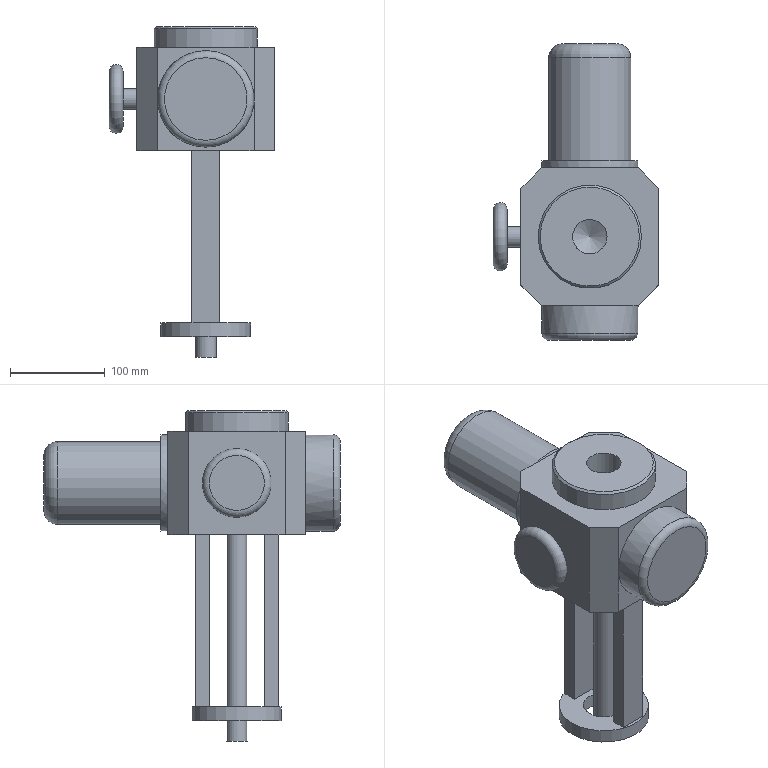Part | NX | features BOSS 6, ABSOLUTE_DATUM_PLANE 3, BLEND 3, DATUM_CSYS 3, HOLE PACKAGE 3, RECT_PAD 3, SIMPLE HOLE 3, SKETCH 3, CHAMFER 2, CYLINDER 2, ABSOLUTE_DATUM_AXIS 1, EXTRUDE 1, SCALE 1 | 1 solid | 49 faces | box 174.546 x 312.729 x 349.093 mm | volume 3776636 mm3 | plane 31 | cylinder 11 | cone 4 | torus 3 | commonest cylinder face diameters 21.818 x2 101.819 x2 14.546 x1 29.091 x1 36.364 x1 43.637 x1
STEP:
#1=CARTESIAN_POINT('',(50.909,-72.728,323.638));
#2=VERTEX_POINT('',#1);
#3=CARTESIAN_POINT('',(-50.909,-72.728,323.638));
#4=VERTEX_POINT('',#3);
#5=CARTESIAN_POINT('',(0.,-72.728,323.638));
#6=DIRECTION('',(0.,-1.,0.));
#7=DIRECTION('',(0.,0.,-1.));
#8=AXIS2_PLACEMENT_3D('',#5,#6,#7);
#9=CIRCLE('',#8,50.909);
#10=EDGE_CURVE('',#2,#4,#9,.T.);
#11=ORIENTED_EDGE('',*,*,#10,.F.);
#12=CARTESIAN_POINT('',(50.909,-72.728,378.184));
#13=VERTEX_POINT('',#12);
#14=CARTESIAN_POINT('',(50.909,-72.728,269.092));
#15=DIRECTION('',(0.,0.,1.));
#16=VECTOR('',#15,1000.);
#17=LINE('',#14,#16);
#18=EDGE_CURVE('',#2,#13,#17,.T.);
#19=ORIENTED_EDGE('',*,*,#18,.T.);
#20=CARTESIAN_POINT('',(-50.909,-72.728,378.184));
#21=VERTEX_POINT('',#20);
#22=CARTESIAN_POINT('',(-72.728,-72.728,378.184));
#23=DIRECTION('',(1.,0.,0.));
#24=VECTOR('',#23,1000.);
#25=LINE('',#22,#24);
#26=EDGE_CURVE('',#21,#13,#25,.T.);
#27=ORIENTED_EDGE('',*,*,#26,.F.);
#28=CARTESIAN_POINT('',(-50.909,-72.728,269.092));
#29=DIRECTION('',(0.,0.,-1.));
#30=VECTOR('',#29,1000.);
#31=LINE('',#28,#30);
#32=EDGE_CURVE('',#21,#4,#31,.T.);
#33=ORIENTED_EDGE('',*,*,#32,.T.);
#34=EDGE_LOOP('',(#11,#19,#27,#33));
#35=FACE_BOUND('',#34,.T.);
#36=CARTESIAN_POINT('',(72.728,-72.728,269.092));
#37=DIRECTION('',(0.,-1.,0.));
#38=DIRECTION('',(0.,0.,-1.));
#39=AXIS2_PLACEMENT_3D('',#36,#37,#38);
#40=PLANE('',#39);
#41=ADVANCED_FACE('',(#35),#40,.T.);
#42=CARTESIAN_POINT('',(50.909,72.728,323.638));
#43=VERTEX_POINT('',#42);
#44=CARTESIAN_POINT('',(-50.909,72.728,323.638));
#45=VERTEX_POINT('',#44);
#46=CARTESIAN_POINT('',(0.,72.728,323.638));
#47=DIRECTION('',(0.,1.,0.));
#48=DIRECTION('',(0.,0.,1.));
#49=AXIS2_PLACEMENT_3D('',#46,#47,#48);
#50=CIRCLE('',#49,50.909);
#51=EDGE_CURVE('',#43,#45,#50,.T.);
#52=ORIENTED_EDGE('',*,*,#51,.F.);
#53=CARTESIAN_POINT('',(50.909,72.728,269.092));
#54=VERTEX_POINT('',#53);
#55=CARTESIAN_POINT('',(50.909,72.728,269.092));
#56=DIRECTION('',(0.,0.,-1.));
#57=VECTOR('',#56,1000.);
#58=LINE('',#55,#57);
#59=EDGE_CURVE('',#43,#54,#58,.T.);
#60=ORIENTED_EDGE('',*,*,#59,.T.);
#61=CARTESIAN_POINT('',(-50.909,72.728,269.092));
#62=VERTEX_POINT('',#61);
#63=CARTESIAN_POINT('',(-72.728,72.728,269.092));
#64=DIRECTION('',(1.,0.,0.));
#65=VECTOR('',#64,1000.);
#66=LINE('',#63,#65);
#67=EDGE_CURVE('',#62,#54,#66,.T.);
#68=ORIENTED_EDGE('',*,*,#67,.F.);
#69=CARTESIAN_POINT('',(-50.909,72.728,269.092));
#70=DIRECTION('',(0.,0.,1.));
#71=VECTOR('',#70,1000.);
#72=LINE('',#69,#71);
#73=EDGE_CURVE('',#62,#45,#72,.T.);
#74=ORIENTED_EDGE('',*,*,#73,.T.);
#75=EDGE_LOOP('',(#52,#60,#68,#74));
#76=FACE_BOUND('',#75,.T.);
#77=CARTESIAN_POINT('',(-72.728,72.728,269.092));
#78=DIRECTION('',(0.,1.,0.));
#79=DIRECTION('',(0.,0.,1.));
#80=AXIS2_PLACEMENT_3D('',#77,#78,#79);
#81=PLANE('',#80);
#82=ADVANCED_FACE('',(#76),#81,.T.);
#83=CARTESIAN_POINT('',(-14.546,-43.637,87.273));
#84=VERTEX_POINT('',#83);
#85=CARTESIAN_POINT('',(-14.546,-29.091,87.273));
#86=VERTEX_POINT('',#85);
#87=CARTESIAN_POINT('',(-14.546,-43.637,87.273));
#88=DIRECTION('',(0.,1.,0.));
#89=VECTOR('',#88,1000.);
#90=LINE('',#87,#89);
#91=EDGE_CURVE('',#84,#86,#90,.T.);
#92=ORIENTED_EDGE('',*,*,#91,.T.);
#93=CARTESIAN_POINT('',(14.546,-29.091,87.273));
#94=VERTEX_POINT('',#93);
#95=CARTESIAN_POINT('',(-14.546,-29.091,87.273));
#96=DIRECTION('',(1.,0.,0.));
#97=VECTOR('',#96,1000.);
#98=LINE('',#95,#97);
#99=EDGE_CURVE('',#86,#94,#98,.T.);
#100=ORIENTED_EDGE('',*,*,#99,.T.);
#101=CARTESIAN_POINT('',(14.546,-43.637,87.273));
#102=VERTEX_POINT('',#101);
#103=CARTESIAN_POINT('',(14.546,-43.637,87.273));
#104=DIRECTION('',(0.,1.,0.));
#105=VECTOR('',#104,1000.);
#106=LINE('',#103,#105);
#107=EDGE_CURVE('',#102,#94,#106,.T.);
#108=ORIENTED_EDGE('',*,*,#107,.F.);
#109=CARTESIAN_POINT('',(-14.546,-43.637,87.273));
#110=DIRECTION('',(1.,0.,0.));
#111=VECTOR('',#110,1000.);
#112=LINE('',#109,#111);
#113=EDGE_CURVE('',#84,#102,#112,.T.);
#114=ORIENTED_EDGE('',*,*,#113,.F.);
#115=EDGE_LOOP('',(#92,#100,#108,#114));
#116=FACE_BOUND('',#115,.T.);
#117=CARTESIAN_POINT('',(-14.546,29.091,87.273));
#118=VERTEX_POINT('',#117);
#119=CARTESIAN_POINT('',(-14.546,43.637,87.273));
#120=VERTEX_POINT('',#119);
#121=CARTESIAN_POINT('',(-14.546,29.091,87.273));
#122=DIRECTION('',(0.,1.,0.));
#123=VECTOR('',#122,1000.);
#124=LINE('',#121,#123);
#125=EDGE_CURVE('',#118,#120,#124,.T.);
#126=ORIENTED_EDGE('',*,*,#125,.T.);
#127=CARTESIAN_POINT('',(14.546,43.637,87.273));
#128=VERTEX_POINT('',#127);
#129=CARTESIAN_POINT('',(-14.546,43.637,87.273));
#130=DIRECTION('',(1.,0.,0.));
#131=VECTOR('',#130,1000.);
#132=LINE('',#129,#131);
#133=EDGE_CURVE('',#120,#128,#132,.T.);
#134=ORIENTED_EDGE('',*,*,#133,.T.);
#135=CARTESIAN_POINT('',(14.546,29.091,87.273));
#136=VERTEX_POINT('',#135);
#137=CARTESIAN_POINT('',(14.546,29.091,87.273));
#138=DIRECTION('',(0.,1.,0.));
#139=VECTOR('',#138,1000.);
#140=LINE('',#137,#139);
#141=EDGE_CURVE('',#136,#128,#140,.T.);
#142=ORIENTED_EDGE('',*,*,#141,.F.);
#143=CARTESIAN_POINT('',(-14.546,29.091,87.273));
#144=DIRECTION('',(1.,0.,0.));
#145=VECTOR('',#144,1000.);
#146=LINE('',#143,#145);
#147=EDGE_CURVE('',#118,#136,#146,.T.);
#148=ORIENTED_EDGE('',*,*,#147,.F.);
#149=EDGE_LOOP('',(#126,#134,#142,#148));
#150=FACE_BOUND('',#149,.T.);
#151=CARTESIAN_POINT('',(21.818,0.,87.273));
#152=VERTEX_POINT('',#151);
#153=CARTESIAN_POINT('',(0.,0.,87.273));
#154=DIRECTION('',(0.,0.,1.));
#155=DIRECTION('',(1.,0.,0.));
#156=AXIS2_PLACEMENT_3D('',#153,#154,#155);
#157=CIRCLE('',#156,21.818);
#158=EDGE_CURVE('',#152,#152,#157,.T.);
#159=ORIENTED_EDGE('',*,*,#158,.F.);
#160=EDGE_LOOP('',(#159));
#161=FACE_BOUND('',#160,.T.);
#162=CARTESIAN_POINT('',(-47.273,0.,87.273));
#163=VERTEX_POINT('',#162);
#164=CARTESIAN_POINT('',(0.,0.,87.273));
#165=DIRECTION('',(0.,0.,-1.));
#166=DIRECTION('',(-1.,0.,0.));
#167=AXIS2_PLACEMENT_3D('',#164,#165,#166);
#168=CIRCLE('',#167,47.273);
#169=EDGE_CURVE('',#163,#163,#168,.T.);
#170=ORIENTED_EDGE('',*,*,#169,.F.);
#171=EDGE_LOOP('',(#170));
#172=FACE_BOUND('',#171,.T.);
#173=CARTESIAN_POINT('',(0.,0.,87.273));
#174=DIRECTION('',(0.,0.,1.));
#175=DIRECTION('',(1.,0.,0.));
#176=AXIS2_PLACEMENT_3D('',#173,#174,#175);
#177=PLANE('',#176);
#178=ADVANCED_FACE('',(#116,#150,#161,#172),#177,.T.);
#179=CARTESIAN_POINT('',(21.818,0.,72.728));
#180=VERTEX_POINT('',#179);
#181=CARTESIAN_POINT('',(0.,0.,72.728));
#182=DIRECTION('',(0.,0.,1.));
#183=DIRECTION('',(1.,0.,0.));
#184=AXIS2_PLACEMENT_3D('',#181,#182,#183);
#185=CIRCLE('',#184,21.818);
#186=EDGE_CURVE('',#180,#180,#185,.T.);
#187=ORIENTED_EDGE('',*,*,#186,.T.);
#188=EDGE_LOOP('',(#187));
#189=FACE_BOUND('',#188,.T.);
#190=CARTESIAN_POINT('',(47.273,0.,72.728));
#191=VERTEX_POINT('',#190);
#192=CARTESIAN_POINT('',(0.,0.,72.728));
#193=DIRECTION('',(0.,0.,1.));
#194=DIRECTION('',(1.,0.,0.));
#195=AXIS2_PLACEMENT_3D('',#192,#193,#194);
#196=CIRCLE('',#195,47.273);
#197=EDGE_CURVE('',#191,#191,#196,.T.);
#198=ORIENTED_EDGE('',*,*,#197,.F.);
#199=EDGE_LOOP('',(#198));
#200=FACE_BOUND('',#199,.T.);
#201=CARTESIAN_POINT('',(0.,0.,72.728));
#202=DIRECTION('',(0.,0.,-1.));
#203=DIRECTION('',(-1.,0.,0.));
#204=AXIS2_PLACEMENT_3D('',#201,#202,#203);
#205=PLANE('',#204);
#206=ADVANCED_FACE('',(#189,#200),#205,.T.);
#207=ORIENTED_EDGE('',*,*,#169,.T.);
#208=EDGE_LOOP('',(#207));
#209=FACE_BOUND('',#208,.T.);
#210=ORIENTED_EDGE('',*,*,#197,.T.);
#211=EDGE_LOOP('',(#210));
#212=FACE_BOUND('',#211,.T.);
#213=CARTESIAN_POINT('',(0.,0.,72.728));
#214=DIRECTION('',(0.,0.,1.));
#215=DIRECTION('',(1.,0.,0.));
#216=AXIS2_PLACEMENT_3D('',#213,#214,#215);
#217=CYLINDRICAL_SURFACE('',#216,47.273);
#218=ADVANCED_FACE('',(#209,#212),#217,.T.);
#219=ORIENTED_EDGE('',*,*,#158,.T.);
#220=EDGE_LOOP('',(#219));
#221=FACE_BOUND('',#220,.T.);
#222=ORIENTED_EDGE('',*,*,#186,.F.);
#223=EDGE_LOOP('',(#222));
#224=FACE_BOUND('',#223,.T.);
#225=CARTESIAN_POINT('',(0.,0.,72.728));
#226=DIRECTION('',(0.,0.,1.));
#227=DIRECTION('',(1.,0.,0.));
#228=AXIS2_PLACEMENT_3D('',#225,#226,#227);
#229=CYLINDRICAL_SURFACE('',#228,21.818);
#230=ADVANCED_FACE('',(#221,#224),#229,.F.);
#231=ORIENTED_EDGE('',*,*,#125,.F.);
#232=CARTESIAN_POINT('',(-14.546,29.091,269.092));
#233=VERTEX_POINT('',#232);
#234=CARTESIAN_POINT('',(-14.546,29.091,269.092));
#235=DIRECTION('',(0.,0.,1.));
#236=VECTOR('',#235,1000.);
#237=LINE('',#234,#236);
#238=EDGE_CURVE('',#118,#233,#237,.T.);
#239=ORIENTED_EDGE('',*,*,#238,.T.);
#240=CARTESIAN_POINT('',(-14.546,43.637,269.092));
#241=VERTEX_POINT('',#240);
#242=CARTESIAN_POINT('',(-14.546,29.091,269.092));
#243=DIRECTION('',(0.,1.,0.));
#244=VECTOR('',#243,1000.);
#245=LINE('',#242,#244);
#246=EDGE_CURVE('',#233,#241,#245,.T.);
#247=ORIENTED_EDGE('',*,*,#246,.T.);
#248=CARTESIAN_POINT('',(-14.546,43.637,269.092));
#249=DIRECTION('',(0.,0.,1.));
#250=VECTOR('',#249,1000.);
#251=LINE('',#248,#250);
#252=EDGE_CURVE('',#120,#241,#251,.T.);
#253=ORIENTED_EDGE('',*,*,#252,.F.);
#254=EDGE_LOOP('',(#231,#239,#247,#253));
#255=FACE_BOUND('',#254,.T.);
#256=CARTESIAN_POINT('',(-14.546,29.091,87.273));
#257=DIRECTION('',(-1.,0.,0.));
#258=DIRECTION('',(0.,0.,1.));
#259=AXIS2_PLACEMENT_3D('',#256,#257,#258);
#260=PLANE('',#259);
#261=ADVANCED_FACE('',(#255),#260,.T.);
#262=ORIENTED_EDGE('',*,*,#133,.F.);
#263=ORIENTED_EDGE('',*,*,#252,.T.);
#264=CARTESIAN_POINT('',(14.546,43.637,269.092));
#265=VERTEX_POINT('',#264);
#266=CARTESIAN_POINT('',(-14.546,43.637,269.092));
#267=DIRECTION('',(1.,0.,0.));
#268=VECTOR('',#267,1000.);
#269=LINE('',#266,#268);
#270=EDGE_CURVE('',#241,#265,#269,.T.);
#271=ORIENTED_EDGE('',*,*,#270,.T.);
#272=CARTESIAN_POINT('',(14.546,43.637,269.092));
#273=DIRECTION('',(0.,0.,1.));
#274=VECTOR('',#273,1000.);
#275=LINE('',#272,#274);
#276=EDGE_CURVE('',#128,#265,#275,.T.);
#277=ORIENTED_EDGE('',*,*,#276,.F.);
#278=EDGE_LOOP('',(#262,#263,#271,#277));
#279=FACE_BOUND('',#278,.T.);
#280=CARTESIAN_POINT('',(-14.546,43.637,87.273));
#281=DIRECTION('',(0.,1.,0.));
#282=DIRECTION('',(0.,0.,1.));
#283=AXIS2_PLACEMENT_3D('',#280,#281,#282);
#284=PLANE('',#283);
#285=ADVANCED_FACE('',(#279),#284,.T.);
#286=ORIENTED_EDGE('',*,*,#141,.T.);
#287=ORIENTED_EDGE('',*,*,#276,.T.);
#288=CARTESIAN_POINT('',(14.546,29.091,269.092));
#289=VERTEX_POINT('',#288);
#290=CARTESIAN_POINT('',(14.546,29.091,269.092));
#291=DIRECTION('',(0.,1.,0.));
#292=VECTOR('',#291,1000.);
#293=LINE('',#290,#292);
#294=EDGE_CURVE('',#289,#265,#293,.T.);
#295=ORIENTED_EDGE('',*,*,#294,.F.);
#296=CARTESIAN_POINT('',(14.546,29.091,269.092));
#297=DIRECTION('',(0.,0.,1.));
#298=VECTOR('',#297,1000.);
#299=LINE('',#296,#298);
#300=EDGE_CURVE('',#136,#289,#299,.T.);
#301=ORIENTED_EDGE('',*,*,#300,.F.);
#302=EDGE_LOOP('',(#286,#287,#295,#301));
#303=FACE_BOUND('',#302,.T.);
#304=CARTESIAN_POINT('',(14.546,43.637,87.273));
#305=DIRECTION('',(1.,0.,0.));
#306=DIRECTION('',(0.,0.,-1.));
#307=AXIS2_PLACEMENT_3D('',#304,#305,#306);
#308=PLANE('',#307);
#309=ADVANCED_FACE('',(#303),#308,.T.);
#310=ORIENTED_EDGE('',*,*,#238,.F.);
#311=ORIENTED_EDGE('',*,*,#147,.T.);
#312=ORIENTED_EDGE('',*,*,#300,.T.);
#313=CARTESIAN_POINT('',(-14.546,29.091,269.092));
#314=DIRECTION('',(1.,0.,0.));
#315=VECTOR('',#314,1000.);
#316=LINE('',#313,#315);
#317=EDGE_CURVE('',#233,#289,#316,.T.);
#318=ORIENTED_EDGE('',*,*,#317,.F.);
#319=EDGE_LOOP('',(#310,#311,#312,#318));
#320=FACE_BOUND('',#319,.T.);
#321=CARTESIAN_POINT('',(14.546,29.091,87.273));
#322=DIRECTION('',(0.,-1.,0.));
#323=DIRECTION('',(0.,0.,-1.));
#324=AXIS2_PLACEMENT_3D('',#321,#322,#323);
#325=PLANE('',#324);
#326=ADVANCED_FACE('',(#320),#325,.T.);
#327=ORIENTED_EDGE('',*,*,#91,.F.);
#328=CARTESIAN_POINT('',(-14.546,-43.637,269.092));
#329=VERTEX_POINT('',#328);
#330=CARTESIAN_POINT('',(-14.546,-43.637,269.092));
#331=DIRECTION('',(0.,0.,1.));
#332=VECTOR('',#331,1000.);
#333=LINE('',#330,#332);
#334=EDGE_CURVE('',#84,#329,#333,.T.);
#335=ORIENTED_EDGE('',*,*,#334,.T.);
#336=CARTESIAN_POINT('',(-14.546,-29.091,269.092));
#337=VERTEX_POINT('',#336);
#338=CARTESIAN_POINT('',(-14.546,-43.637,269.092));
#339=DIRECTION('',(0.,1.,0.));
#340=VECTOR('',#339,1000.);
#341=LINE('',#338,#340);
#342=EDGE_CURVE('',#329,#337,#341,.T.);
#343=ORIENTED_EDGE('',*,*,#342,.T.);
#344=CARTESIAN_POINT('',(-14.546,-29.091,269.092));
#345=DIRECTION('',(0.,0.,1.));
#346=VECTOR('',#345,1000.);
#347=LINE('',#344,#346);
#348=EDGE_CURVE('',#86,#337,#347,.T.);
#349=ORIENTED_EDGE('',*,*,#348,.F.);
#350=EDGE_LOOP('',(#327,#335,#343,#349));
#351=FACE_BOUND('',#350,.T.);
#352=CARTESIAN_POINT('',(-14.546,-43.637,87.273));
#353=DIRECTION('',(-1.,0.,0.));
#354=DIRECTION('',(0.,0.,1.));
#355=AXIS2_PLACEMENT_3D('',#352,#353,#354);
#356=PLANE('',#355);
#357=ADVANCED_FACE('',(#351),#356,.T.);
#358=ORIENTED_EDGE('',*,*,#99,.F.);
#359=ORIENTED_EDGE('',*,*,#348,.T.);
#360=CARTESIAN_POINT('',(14.546,-29.091,269.092));
#361=VERTEX_POINT('',#360);
#362=CARTESIAN_POINT('',(-14.546,-29.091,269.092));
#363=DIRECTION('',(1.,0.,0.));
#364=VECTOR('',#363,1000.);
#365=LINE('',#362,#364);
#366=EDGE_CURVE('',#337,#361,#365,.T.);
#367=ORIENTED_EDGE('',*,*,#366,.T.);
#368=CARTESIAN_POINT('',(14.546,-29.091,269.092));
#369=DIRECTION('',(0.,0.,1.));
#370=VECTOR('',#369,1000.);
#371=LINE('',#368,#370);
#372=EDGE_CURVE('',#94,#361,#371,.T.);
#373=ORIENTED_EDGE('',*,*,#372,.F.);
#374=EDGE_LOOP('',(#358,#359,#367,#373));
#375=FACE_BOUND('',#374,.T.);
#376=CARTESIAN_POINT('',(-14.546,-29.091,87.273));
#377=DIRECTION('',(0.,1.,0.));
#378=DIRECTION('',(0.,0.,1.));
#379=AXIS2_PLACEMENT_3D('',#376,#377,#378);
#380=PLANE('',#379);
#381=ADVANCED_FACE('',(#375),#380,.T.);
#382=ORIENTED_EDGE('',*,*,#107,.T.);
#383=ORIENTED_EDGE('',*,*,#372,.T.);
#384=CARTESIAN_POINT('',(14.546,-43.637,269.092));
#385=VERTEX_POINT('',#384);
#386=CARTESIAN_POINT('',(14.546,-43.637,269.092));
#387=DIRECTION('',(0.,1.,0.));
#388=VECTOR('',#387,1000.);
#389=LINE('',#386,#388);
#390=EDGE_CURVE('',#385,#361,#389,.T.);
#391=ORIENTED_EDGE('',*,*,#390,.F.);
#392=CARTESIAN_POINT('',(14.546,-43.637,269.092));
#393=DIRECTION('',(0.,0.,1.));
#394=VECTOR('',#393,1000.);
#395=LINE('',#392,#394);
#396=EDGE_CURVE('',#102,#385,#395,.T.);
#397=ORIENTED_EDGE('',*,*,#396,.F.);
#398=EDGE_LOOP('',(#382,#383,#391,#397));
#399=FACE_BOUND('',#398,.T.);
#400=CARTESIAN_POINT('',(14.546,-29.091,87.273));
#401=DIRECTION('',(1.,0.,0.));
#402=DIRECTION('',(0.,0.,-1.));
#403=AXIS2_PLACEMENT_3D('',#400,#401,#402);
#404=PLANE('',#403);
#405=ADVANCED_FACE('',(#399),#404,.T.);
#406=ORIENTED_EDGE('',*,*,#334,.F.);
#407=ORIENTED_EDGE('',*,*,#113,.T.);
#408=ORIENTED_EDGE('',*,*,#396,.T.);
#409=CARTESIAN_POINT('',(-14.546,-43.637,269.092));
#410=DIRECTION('',(1.,0.,0.));
#411=VECTOR('',#410,1000.);
#412=LINE('',#409,#411);
#413=EDGE_CURVE('',#329,#385,#412,.T.);
#414=ORIENTED_EDGE('',*,*,#413,.F.);
#415=EDGE_LOOP('',(#406,#407,#408,#414));
#416=FACE_BOUND('',#415,.T.);
#417=CARTESIAN_POINT('',(14.546,-43.637,87.273));
#418=DIRECTION('',(0.,-1.,0.));
#419=DIRECTION('',(0.,0.,-1.));
#420=AXIS2_PLACEMENT_3D('',#417,#418,#419);
#421=PLANE('',#420);
#422=ADVANCED_FACE('',(#416),#421,.T.);
#423=CARTESIAN_POINT('',(-72.728,0.,334.547));
#424=VERTEX_POINT('',#423);
#425=CARTESIAN_POINT('',(-72.728,0.,323.638));
#426=DIRECTION('',(-1.,0.,0.));
#427=DIRECTION('',(0.,0.,1.));
#428=AXIS2_PLACEMENT_3D('',#425,#426,#427);
#429=CIRCLE('',#428,10.909);
#430=EDGE_CURVE('',#424,#424,#429,.T.);
#431=ORIENTED_EDGE('',*,*,#430,.F.);
#432=EDGE_LOOP('',(#431));
#433=FACE_BOUND('',#432,.T.);
#434=CARTESIAN_POINT('',(-72.728,-50.909,378.184));
#435=VERTEX_POINT('',#434);
#436=CARTESIAN_POINT('',(-72.728,50.909,378.184));
#437=VERTEX_POINT('',#436);
#438=CARTESIAN_POINT('',(-72.728,-72.728,378.184));
#439=DIRECTION('',(0.,1.,0.));
#440=VECTOR('',#439,1000.);
#441=LINE('',#438,#440);
#442=EDGE_CURVE('',#435,#437,#441,.T.);
#443=ORIENTED_EDGE('',*,*,#442,.T.);
#444=CARTESIAN_POINT('',(-72.728,50.909,269.092));
#445=VERTEX_POINT('',#444);
#446=CARTESIAN_POINT('',(-72.728,50.909,269.092));
#447=DIRECTION('',(0.,0.,-1.));
#448=VECTOR('',#447,1000.);
#449=LINE('',#446,#448);
#450=EDGE_CURVE('',#437,#445,#449,.T.);
#451=ORIENTED_EDGE('',*,*,#450,.T.);
#452=CARTESIAN_POINT('',(-72.728,-50.909,269.092));
#453=VERTEX_POINT('',#452);
#454=CARTESIAN_POINT('',(-72.728,-72.728,269.092));
#455=DIRECTION('',(0.,1.,0.));
#456=VECTOR('',#455,1000.);
#457=LINE('',#454,#456);
#458=EDGE_CURVE('',#453,#445,#457,.T.);
#459=ORIENTED_EDGE('',*,*,#458,.F.);
#460=CARTESIAN_POINT('',(-72.728,-50.909,269.092));
#461=DIRECTION('',(0.,0.,1.));
#462=VECTOR('',#461,1000.);
#463=LINE('',#460,#462);
#464=EDGE_CURVE('',#453,#435,#463,.T.);
#465=ORIENTED_EDGE('',*,*,#464,.T.);
#466=EDGE_LOOP('',(#443,#451,#459,#465));
#467=FACE_BOUND('',#466,.T.);
#468=CARTESIAN_POINT('',(-72.728,-72.728,269.092));
#469=DIRECTION('',(-1.,0.,0.));
#470=DIRECTION('',(0.,0.,1.));
#471=AXIS2_PLACEMENT_3D('',#468,#469,#470);
#472=PLANE('',#471);
#473=ADVANCED_FACE('',(#433,#467),#472,.T.);
#474=CARTESIAN_POINT('',(0.,72.728,323.638));
#475=DIRECTION('',(0.,1.,0.));
#476=DIRECTION('',(0.,0.,1.));
#477=AXIS2_PLACEMENT_3D('',#474,#475,#476);
#478=CIRCLE('',#477,50.909);
#479=EDGE_CURVE('',#45,#43,#478,.T.);
#480=ORIENTED_EDGE('',*,*,#479,.F.);
#481=CARTESIAN_POINT('',(-50.909,72.728,378.184));
#482=VERTEX_POINT('',#481);
#483=CARTESIAN_POINT('',(-50.909,72.728,269.092));
#484=DIRECTION('',(0.,0.,1.));
#485=VECTOR('',#484,1000.);
#486=LINE('',#483,#485);
#487=EDGE_CURVE('',#45,#482,#486,.T.);
#488=ORIENTED_EDGE('',*,*,#487,.T.);
#489=CARTESIAN_POINT('',(50.909,72.728,378.184));
#490=VERTEX_POINT('',#489);
#491=CARTESIAN_POINT('',(-72.728,72.728,378.184));
#492=DIRECTION('',(1.,0.,0.));
#493=VECTOR('',#492,1000.);
#494=LINE('',#491,#493);
#495=EDGE_CURVE('',#482,#490,#494,.T.);
#496=ORIENTED_EDGE('',*,*,#495,.T.);
#497=CARTESIAN_POINT('',(50.909,72.728,269.092));
#498=DIRECTION('',(0.,0.,-1.));
#499=VECTOR('',#498,1000.);
#500=LINE('',#497,#499);
#501=EDGE_CURVE('',#490,#43,#500,.T.);
#502=ORIENTED_EDGE('',*,*,#501,.T.);
#503=EDGE_LOOP('',(#480,#488,#496,#502));
#504=FACE_BOUND('',#503,.T.);
#505=CARTESIAN_POINT('',(-72.728,72.728,269.092));
#506=DIRECTION('',(0.,1.,0.));
#507=DIRECTION('',(0.,0.,1.));
#508=AXIS2_PLACEMENT_3D('',#505,#506,#507);
#509=PLANE('',#508);
#510=ADVANCED_FACE('',(#504),#509,.T.);
#511=CARTESIAN_POINT('',(72.728,-50.909,269.092));
#512=VERTEX_POINT('',#511);
#513=CARTESIAN_POINT('',(72.728,50.909,269.092));
#514=VERTEX_POINT('',#513);
#515=CARTESIAN_POINT('',(72.728,-72.728,269.092));
#516=DIRECTION('',(0.,1.,0.));
#517=VECTOR('',#516,1000.);
#518=LINE('',#515,#517);
#519=EDGE_CURVE('',#512,#514,#518,.T.);
#520=ORIENTED_EDGE('',*,*,#519,.T.);
#521=CARTESIAN_POINT('',(72.728,50.909,378.184));
#522=VERTEX_POINT('',#521);
#523=CARTESIAN_POINT('',(72.728,50.909,269.092));
#524=DIRECTION('',(0.,0.,1.));
#525=VECTOR('',#524,1000.);
#526=LINE('',#523,#525);
#527=EDGE_CURVE('',#514,#522,#526,.T.);
#528=ORIENTED_EDGE('',*,*,#527,.T.);
#529=CARTESIAN_POINT('',(72.728,-50.909,378.184));
#530=VERTEX_POINT('',#529);
#531=CARTESIAN_POINT('',(72.728,-72.728,378.184));
#532=DIRECTION('',(0.,1.,0.));
#533=VECTOR('',#532,1000.);
#534=LINE('',#531,#533);
#535=EDGE_CURVE('',#530,#522,#534,.T.);
#536=ORIENTED_EDGE('',*,*,#535,.F.);
#537=CARTESIAN_POINT('',(72.728,-50.909,269.092));
#538=DIRECTION('',(0.,0.,-1.));
#539=VECTOR('',#538,1000.);
#540=LINE('',#537,#539);
#541=EDGE_CURVE('',#530,#512,#540,.T.);
#542=ORIENTED_EDGE('',*,*,#541,.T.);
#543=EDGE_LOOP('',(#520,#528,#536,#542));
#544=FACE_BOUND('',#543,.T.);
#545=CARTESIAN_POINT('',(72.728,72.728,269.092));
#546=DIRECTION('',(1.,0.,0.));
#547=DIRECTION('',(0.,0.,-1.));
#548=AXIS2_PLACEMENT_3D('',#545,#546,#547);
#549=PLANE('',#548);
#550=ADVANCED_FACE('',(#544),#549,.T.);
#551=CARTESIAN_POINT('',(-10.909,0.,269.092));
#552=VERTEX_POINT('',#551);
#553=CARTESIAN_POINT('',(0.,0.,269.092));
#554=DIRECTION('',(0.,0.,-1.));
#555=DIRECTION('',(-1.,0.,0.));
#556=AXIS2_PLACEMENT_3D('',#553,#554,#555);
#557=CIRCLE('',#556,10.909);
#558=EDGE_CURVE('',#552,#552,#557,.T.);
#559=ORIENTED_EDGE('',*,*,#558,.F.);
#560=EDGE_LOOP('',(#559));
#561=FACE_BOUND('',#560,.T.);
#562=ORIENTED_EDGE('',*,*,#270,.F.);
#563=ORIENTED_EDGE('',*,*,#246,.F.);
#564=ORIENTED_EDGE('',*,*,#317,.T.);
#565=ORIENTED_EDGE('',*,*,#294,.T.);
#566=EDGE_LOOP('',(#562,#563,#564,#565));
#567=FACE_BOUND('',#566,.T.);
#568=ORIENTED_EDGE('',*,*,#366,.F.);
#569=ORIENTED_EDGE('',*,*,#342,.F.);
#570=ORIENTED_EDGE('',*,*,#413,.T.);
#571=ORIENTED_EDGE('',*,*,#390,.T.);
#572=EDGE_LOOP('',(#568,#569,#570,#571));
#573=FACE_BOUND('',#572,.T.);
#574=ORIENTED_EDGE('',*,*,#67,.T.);
#575=CARTESIAN_POINT('',(134.546,-10.909,269.092));
#576=DIRECTION('',(-0.7071,0.7071,0.));
#577=VECTOR('',#576,1000.);
#578=LINE('',#575,#577);
#579=EDGE_CURVE('',#54,#514,#578,.F.);
#580=ORIENTED_EDGE('',*,*,#579,.T.);
#581=ORIENTED_EDGE('',*,*,#519,.F.);
#582=CARTESIAN_POINT('',(50.909,-72.728,269.092));
#583=VERTEX_POINT('',#582);
#584=CARTESIAN_POINT('',(61.819,-61.819,269.092));
#585=DIRECTION('',(0.7071,0.7071,0.));
#586=VECTOR('',#585,1000.);
#587=LINE('',#584,#586);
#588=EDGE_CURVE('',#512,#583,#587,.F.);
#589=ORIENTED_EDGE('',*,*,#588,.T.);
#590=CARTESIAN_POINT('',(-50.909,-72.728,269.092));
#591=VERTEX_POINT('',#590);
#592=CARTESIAN_POINT('',(-72.728,-72.728,269.092));
#593=DIRECTION('',(1.,0.,0.));
#594=VECTOR('',#593,1000.);
#595=LINE('',#592,#594);
#596=EDGE_CURVE('',#591,#583,#595,.T.);
#597=ORIENTED_EDGE('',*,*,#596,.F.);
#598=CARTESIAN_POINT('',(10.909,-134.546,269.092));
#599=DIRECTION('',(0.7071,-0.7071,0.));
#600=VECTOR('',#599,1000.);
#601=LINE('',#598,#600);
#602=EDGE_CURVE('',#591,#453,#601,.F.);
#603=ORIENTED_EDGE('',*,*,#602,.T.);
#604=ORIENTED_EDGE('',*,*,#458,.T.);
#605=CARTESIAN_POINT('',(-61.819,61.819,269.092));
#606=DIRECTION('',(-0.7071,-0.7071,0.));
#607=VECTOR('',#606,1000.);
#608=LINE('',#605,#607);
#609=EDGE_CURVE('',#445,#62,#608,.F.);
#610=ORIENTED_EDGE('',*,*,#609,.T.);
#611=EDGE_LOOP('',(#574,#580,#581,#589,#597,#603,#604,#610));
#612=FACE_BOUND('',#611,.T.);
#613=CARTESIAN_POINT('',(72.728,-72.728,269.092));
#614=DIRECTION('',(0.,0.,-1.));
#615=DIRECTION('',(-1.,0.,0.));
#616=AXIS2_PLACEMENT_3D('',#613,#614,#615);
#617=PLANE('',#616);
#618=ADVANCED_FACE('',(#561,#567,#573,#612),#617,.T.);
#619=CARTESIAN_POINT('',(0.,-72.728,323.638));
#620=DIRECTION('',(0.,-1.,0.));
#621=DIRECTION('',(0.,0.,-1.));
#622=AXIS2_PLACEMENT_3D('',#619,#620,#621);
#623=CIRCLE('',#622,50.909);
#624=EDGE_CURVE('',#4,#2,#623,.T.);
#625=ORIENTED_EDGE('',*,*,#624,.F.);
#626=CARTESIAN_POINT('',(-50.909,-72.728,269.092));
#627=DIRECTION('',(0.,0.,-1.));
#628=VECTOR('',#627,1000.);
#629=LINE('',#626,#628);
#630=EDGE_CURVE('',#4,#591,#629,.T.);
#631=ORIENTED_EDGE('',*,*,#630,.T.);
#632=ORIENTED_EDGE('',*,*,#596,.T.);
#633=CARTESIAN_POINT('',(50.909,-72.728,269.092));
#634=DIRECTION('',(0.,0.,1.));
#635=VECTOR('',#634,1000.);
#636=LINE('',#633,#635);
#637=EDGE_CURVE('',#583,#2,#636,.T.);
#638=ORIENTED_EDGE('',*,*,#637,.T.);
#639=EDGE_LOOP('',(#625,#631,#632,#638));
#640=FACE_BOUND('',#639,.T.);
#641=CARTESIAN_POINT('',(72.728,-72.728,269.092));
#642=DIRECTION('',(0.,-1.,0.));
#643=DIRECTION('',(0.,0.,-1.));
#644=AXIS2_PLACEMENT_3D('',#641,#642,#643);
#645=PLANE('',#644);
#646=ADVANCED_FACE('',(#640),#645,.T.);
#647=CARTESIAN_POINT('',(54.546,0.,378.184));
#648=VERTEX_POINT('',#647);
#649=CARTESIAN_POINT('',(0.,0.,378.184));
#650=DIRECTION('',(0.,0.,1.));
#651=DIRECTION('',(1.,0.,0.));
#652=AXIS2_PLACEMENT_3D('',#649,#650,#651);
#653=CIRCLE('',#652,54.546);
#654=EDGE_CURVE('',#648,#648,#653,.T.);
#655=ORIENTED_EDGE('',*,*,#654,.F.);
#656=EDGE_LOOP('',(#655));
#657=FACE_BOUND('',#656,.T.);
#658=ORIENTED_EDGE('',*,*,#535,.T.);
#659=CARTESIAN_POINT('',(61.819,61.819,378.184));
#660=DIRECTION('',(0.7071,-0.7071,0.));
#661=VECTOR('',#660,1000.);
#662=LINE('',#659,#661);
#663=EDGE_CURVE('',#522,#490,#662,.F.);
#664=ORIENTED_EDGE('',*,*,#663,.T.);
#665=ORIENTED_EDGE('',*,*,#495,.F.);
#666=CARTESIAN_POINT('',(-134.546,-10.909,378.184));
#667=DIRECTION('',(0.7071,0.7071,0.));
#668=VECTOR('',#667,1000.);
#669=LINE('',#666,#668);
#670=EDGE_CURVE('',#482,#437,#669,.F.);
#671=ORIENTED_EDGE('',*,*,#670,.T.);
#672=ORIENTED_EDGE('',*,*,#442,.F.);
#673=CARTESIAN_POINT('',(-61.819,-61.819,378.184));
#674=DIRECTION('',(-0.7071,0.7071,0.));
#675=VECTOR('',#674,1000.);
#676=LINE('',#673,#675);
#677=EDGE_CURVE('',#435,#21,#676,.F.);
#678=ORIENTED_EDGE('',*,*,#677,.T.);
#679=ORIENTED_EDGE('',*,*,#26,.T.);
#680=CARTESIAN_POINT('',(-10.909,-134.546,378.184));
#681=DIRECTION('',(-0.7071,-0.7071,0.));
#682=VECTOR('',#681,1000.);
#683=LINE('',#680,#682);
#684=EDGE_CURVE('',#13,#530,#683,.F.);
#685=ORIENTED_EDGE('',*,*,#684,.T.);
#686=EDGE_LOOP('',(#658,#664,#665,#671,#672,#678,#679,#685));
#687=FACE_BOUND('',#686,.T.);
#688=CARTESIAN_POINT('',(-72.728,-72.728,378.184));
#689=DIRECTION('',(0.,0.,1.));
#690=DIRECTION('',(1.,0.,0.));
#691=AXIS2_PLACEMENT_3D('',#688,#689,#690);
#692=PLANE('',#691);
#693=ADVANCED_FACE('',(#657,#687),#692,.T.);
#694=ORIENTED_EDGE('',*,*,#579,.F.);
#695=ORIENTED_EDGE('',*,*,#59,.F.);
#696=ORIENTED_EDGE('',*,*,#501,.F.);
#697=ORIENTED_EDGE('',*,*,#663,.F.);
#698=ORIENTED_EDGE('',*,*,#527,.F.);
#699=EDGE_LOOP('',(#694,#695,#696,#697,#698));
#700=FACE_BOUND('',#699,.T.);
#701=CARTESIAN_POINT('',(72.728,50.909,269.092));
#702=DIRECTION('',(-0.7071,-0.7071,0.));
#703=DIRECTION('',(0.7071,-0.7071,0.));
#704=AXIS2_PLACEMENT_3D('',#701,#702,#703);
#705=PLANE('',#704);
#706=ADVANCED_FACE('',(#700),#705,.F.);
#707=ORIENTED_EDGE('',*,*,#609,.F.);
#708=ORIENTED_EDGE('',*,*,#450,.F.);
#709=ORIENTED_EDGE('',*,*,#670,.F.);
#710=ORIENTED_EDGE('',*,*,#487,.F.);
#711=ORIENTED_EDGE('',*,*,#73,.F.);
#712=EDGE_LOOP('',(#707,#708,#709,#710,#711));
#713=FACE_BOUND('',#712,.T.);
#714=CARTESIAN_POINT('',(-50.909,72.728,269.092));
#715=DIRECTION('',(0.7071,-0.7071,0.));
#716=DIRECTION('',(0.7071,0.7071,0.));
#717=AXIS2_PLACEMENT_3D('',#714,#715,#716);
#718=PLANE('',#717);
#719=ADVANCED_FACE('',(#713),#718,.F.);
#720=ORIENTED_EDGE('',*,*,#588,.F.);
#721=ORIENTED_EDGE('',*,*,#541,.F.);
#722=ORIENTED_EDGE('',*,*,#684,.F.);
#723=ORIENTED_EDGE('',*,*,#18,.F.);
#724=ORIENTED_EDGE('',*,*,#637,.F.);
#725=EDGE_LOOP('',(#720,#721,#722,#723,#724));
#726=FACE_BOUND('',#725,.T.);
#727=CARTESIAN_POINT('',(50.909,-72.728,269.092));
#728=DIRECTION('',(-0.7071,0.7071,0.));
#729=DIRECTION('',(-0.7071,-0.7071,0.));
#730=AXIS2_PLACEMENT_3D('',#727,#728,#729);
#731=PLANE('',#730);
#732=ADVANCED_FACE('',(#726),#731,.F.);
#733=ORIENTED_EDGE('',*,*,#602,.F.);
#734=ORIENTED_EDGE('',*,*,#630,.F.);
#735=ORIENTED_EDGE('',*,*,#32,.F.);
#736=ORIENTED_EDGE('',*,*,#677,.F.);
#737=ORIENTED_EDGE('',*,*,#464,.F.);
#738=EDGE_LOOP('',(#733,#734,#735,#736,#737));
#739=FACE_BOUND('',#738,.T.);
#740=CARTESIAN_POINT('',(-72.728,-50.909,269.092));
#741=DIRECTION('',(0.7071,0.7071,0.));
#742=DIRECTION('',(-0.7071,0.7071,0.));
#743=AXIS2_PLACEMENT_3D('',#740,#741,#742);
#744=PLANE('',#743);
#745=ADVANCED_FACE('',(#739),#744,.F.);
#746=CARTESIAN_POINT('',(-18.182,0.,400.002));
#747=VERTEX_POINT('',#746);
#748=CARTESIAN_POINT('',(0.,0.,400.002));
#749=DIRECTION('',(0.,0.,-1.));
#750=DIRECTION('',(-1.,0.,0.));
#751=AXIS2_PLACEMENT_3D('',#748,#749,#750);
#752=CIRCLE('',#751,18.182);
#753=EDGE_CURVE('',#747,#747,#752,.T.);
#754=ORIENTED_EDGE('',*,*,#753,.T.);
#755=EDGE_LOOP('',(#754));
#756=FACE_BOUND('',#755,.T.);
#757=CARTESIAN_POINT('',(52.364,0.,400.002));
#758=VERTEX_POINT('',#757);
#759=CARTESIAN_POINT('',(0.,0.,400.002));
#760=DIRECTION('',(0.,0.,1.));
#761=DIRECTION('',(1.,0.,0.));
#762=AXIS2_PLACEMENT_3D('',#759,#760,#761);
#763=CIRCLE('',#762,52.364);
#764=EDGE_CURVE('',#758,#758,#763,.T.);
#765=ORIENTED_EDGE('',*,*,#764,.T.);
#766=EDGE_LOOP('',(#765));
#767=FACE_BOUND('',#766,.T.);
#768=CARTESIAN_POINT('',(0.,0.,400.002));
#769=DIRECTION('',(0.,0.,1.));
#770=DIRECTION('',(1.,0.,0.));
#771=AXIS2_PLACEMENT_3D('',#768,#769,#770);
#772=PLANE('',#771);
#773=ADVANCED_FACE('',(#756,#767),#772,.T.);
#774=CARTESIAN_POINT('',(54.546,0.,397.82));
#775=VERTEX_POINT('',#774);
#776=CARTESIAN_POINT('',(0.,0.,397.82));
#777=DIRECTION('',(0.,0.,1.));
#778=DIRECTION('',(1.,0.,0.));
#779=AXIS2_PLACEMENT_3D('',#776,#777,#778);
#780=CIRCLE('',#779,54.546);
#781=EDGE_CURVE('',#775,#775,#780,.F.);
#782=ORIENTED_EDGE('',*,*,#781,.T.);
#783=EDGE_LOOP('',(#782));
#784=FACE_BOUND('',#783,.T.);
#785=ORIENTED_EDGE('',*,*,#654,.T.);
#786=EDGE_LOOP('',(#785));
#787=FACE_BOUND('',#786,.T.);
#788=CARTESIAN_POINT('',(0.,0.,378.184));
#789=DIRECTION('',(0.,0.,1.));
#790=DIRECTION('',(1.,0.,0.));
#791=AXIS2_PLACEMENT_3D('',#788,#789,#790);
#792=CYLINDRICAL_SURFACE('',#791,54.546);
#793=ADVANCED_FACE('',(#784,#787),#792,.T.);
#794=CARTESIAN_POINT('',(0.,80.,374.548));
#795=VERTEX_POINT('',#794);
#796=CARTESIAN_POINT('',(0.,80.,323.638));
#797=DIRECTION('',(0.,1.,0.));
#798=DIRECTION('',(0.,0.,1.));
#799=AXIS2_PLACEMENT_3D('',#796,#797,#798);
#800=CIRCLE('',#799,50.909);
#801=EDGE_CURVE('',#795,#795,#800,.T.);
#802=ORIENTED_EDGE('',*,*,#801,.T.);
#803=EDGE_LOOP('',(#802));
#804=FACE_BOUND('',#803,.T.);
#805=CARTESIAN_POINT('',(0.,80.,280.002));
#806=VERTEX_POINT('',#805);
#807=CARTESIAN_POINT('',(0.,80.,323.638));
#808=DIRECTION('',(0.,-1.,0.));
#809=DIRECTION('',(0.,0.,-1.));
#810=AXIS2_PLACEMENT_3D('',#807,#808,#809);
#811=CIRCLE('',#810,43.637);
#812=EDGE_CURVE('',#806,#806,#811,.T.);
#813=ORIENTED_EDGE('',*,*,#812,.T.);
#814=EDGE_LOOP('',(#813));
#815=FACE_BOUND('',#814,.T.);
#816=CARTESIAN_POINT('',(0.,80.,323.638));
#817=DIRECTION('',(0.,-1.,0.));
#818=DIRECTION('',(0.,0.,-1.));
#819=AXIS2_PLACEMENT_3D('',#816,#817,#818);
#820=PLANE('',#819);
#821=ADVANCED_FACE('',(#804,#815),#820,.F.);
#822=ORIENTED_EDGE('',*,*,#51,.T.);
#823=ORIENTED_EDGE('',*,*,#479,.T.);
#824=EDGE_LOOP('',(#822,#823));
#825=FACE_BOUND('',#824,.T.);
#826=ORIENTED_EDGE('',*,*,#801,.F.);
#827=EDGE_LOOP('',(#826));
#828=FACE_BOUND('',#827,.T.);
#829=CARTESIAN_POINT('',(0.,72.728,323.638));
#830=DIRECTION('',(0.,1.,0.));
#831=DIRECTION('',(0.,0.,1.));
#832=AXIS2_PLACEMENT_3D('',#829,#830,#831);
#833=CYLINDRICAL_SURFACE('',#832,50.909);
#834=ADVANCED_FACE('',(#825,#828),#833,.T.);
#835=CARTESIAN_POINT('',(0.,203.638,352.729));
#836=VERTEX_POINT('',#835);
#837=CARTESIAN_POINT('',(0.,203.638,323.638));
#838=DIRECTION('',(0.,1.,0.));
#839=DIRECTION('',(0.,0.,1.));
#840=AXIS2_PLACEMENT_3D('',#837,#838,#839);
#841=CIRCLE('',#840,29.091);
#842=EDGE_CURVE('',#836,#836,#841,.T.);
#843=ORIENTED_EDGE('',*,*,#842,.T.);
#844=EDGE_LOOP('',(#843));
#845=FACE_BOUND('',#844,.T.);
#846=CARTESIAN_POINT('',(0.,203.638,323.638));
#847=DIRECTION('',(0.,1.,0.));
#848=DIRECTION('',(0.,0.,1.));
#849=AXIS2_PLACEMENT_3D('',#846,#847,#848);
#850=PLANE('',#849);
#851=ADVANCED_FACE('',(#845),#850,.T.);
#852=CARTESIAN_POINT('',(0.,189.092,367.275));
#853=VERTEX_POINT('',#852);
#854=CARTESIAN_POINT('',(0.,189.092,323.638));
#855=DIRECTION('',(0.,1.,0.));
#856=DIRECTION('',(0.,0.,1.));
#857=AXIS2_PLACEMENT_3D('',#854,#855,#856);
#858=CIRCLE('',#857,43.637);
#859=EDGE_CURVE('',#853,#853,#858,.F.);
#860=ORIENTED_EDGE('',*,*,#859,.F.);
#861=EDGE_LOOP('',(#860));
#862=FACE_BOUND('',#861,.T.);
#863=ORIENTED_EDGE('',*,*,#842,.F.);
#864=EDGE_LOOP('',(#863));
#865=FACE_BOUND('',#864,.T.);
#866=CARTESIAN_POINT('',(0.,189.092,323.638));
#867=DIRECTION('',(0.,1.,0.));
#868=DIRECTION('',(0.,0.,1.));
#869=AXIS2_PLACEMENT_3D('',#866,#867,#868);
#870=TOROIDAL_SURFACE('',#869,29.091,14.546);
#871=ADVANCED_FACE('',(#862,#865),#870,.T.);
#872=ORIENTED_EDGE('',*,*,#812,.F.);
#873=EDGE_LOOP('',(#872));
#874=FACE_BOUND('',#873,.T.);
#875=ORIENTED_EDGE('',*,*,#859,.T.);
#876=EDGE_LOOP('',(#875));
#877=FACE_BOUND('',#876,.T.);
#878=CARTESIAN_POINT('',(0.,72.728,323.638));
#879=DIRECTION('',(0.,1.,0.));
#880=DIRECTION('',(0.,0.,1.));
#881=AXIS2_PLACEMENT_3D('',#878,#879,#880);
#882=CYLINDRICAL_SURFACE('',#881,43.637);
#883=ADVANCED_FACE('',(#874,#877),#882,.T.);
#884=CARTESIAN_POINT('',(0.,-109.092,280.002));
#885=VERTEX_POINT('',#884);
#886=CARTESIAN_POINT('',(0.,-109.092,323.638));
#887=DIRECTION('',(0.,-1.,0.));
#888=DIRECTION('',(0.,0.,-1.));
#889=AXIS2_PLACEMENT_3D('',#886,#887,#888);
#890=CIRCLE('',#889,43.637);
#891=EDGE_CURVE('',#885,#885,#890,.T.);
#892=ORIENTED_EDGE('',*,*,#891,.T.);
#893=EDGE_LOOP('',(#892));
#894=FACE_BOUND('',#893,.T.);
#895=CARTESIAN_POINT('',(0.,-109.092,323.638));
#896=DIRECTION('',(0.,-1.,0.));
#897=DIRECTION('',(0.,0.,-1.));
#898=AXIS2_PLACEMENT_3D('',#895,#896,#897);
#899=PLANE('',#898);
#900=ADVANCED_FACE('',(#894),#899,.T.);
#901=CARTESIAN_POINT('',(0.,-101.819,272.729));
#902=VERTEX_POINT('',#901);
#903=CARTESIAN_POINT('',(0.,-101.819,323.638));
#904=DIRECTION('',(0.,-1.,0.));
#905=DIRECTION('',(0.,0.,-1.));
#906=AXIS2_PLACEMENT_3D('',#903,#904,#905);
#907=CIRCLE('',#906,50.909);
#908=EDGE_CURVE('',#902,#902,#907,.F.);
#909=ORIENTED_EDGE('',*,*,#908,.T.);
#910=EDGE_LOOP('',(#909));
#911=FACE_BOUND('',#910,.T.);
#912=ORIENTED_EDGE('',*,*,#10,.T.);
#913=ORIENTED_EDGE('',*,*,#624,.T.);
#914=EDGE_LOOP('',(#912,#913));
#915=FACE_BOUND('',#914,.T.);
#916=CARTESIAN_POINT('',(0.,-72.728,323.638));
#917=DIRECTION('',(0.,-1.,0.));
#918=DIRECTION('',(0.,0.,-1.));
#919=AXIS2_PLACEMENT_3D('',#916,#917,#918);
#920=CYLINDRICAL_SURFACE('',#919,50.909);
#921=ADVANCED_FACE('',(#911,#915),#920,.T.);
#922=ORIENTED_EDGE('',*,*,#908,.F.);
#923=EDGE_LOOP('',(#922));
#924=FACE_BOUND('',#923,.T.);
#925=ORIENTED_EDGE('',*,*,#891,.F.);
#926=EDGE_LOOP('',(#925));
#927=FACE_BOUND('',#926,.T.);
#928=CARTESIAN_POINT('',(0.,-101.819,323.638));
#929=DIRECTION('',(0.,-1.,0.));
#930=DIRECTION('',(0.,0.,-1.));
#931=AXIS2_PLACEMENT_3D('',#928,#929,#930);
#932=TOROIDAL_SURFACE('',#931,43.637,7.273);
#933=ADVANCED_FACE('',(#924,#927),#932,.T.);
#934=ORIENTED_EDGE('',*,*,#781,.F.);
#935=EDGE_LOOP('',(#934));
#936=FACE_BOUND('',#935,.T.);
#937=ORIENTED_EDGE('',*,*,#764,.F.);
#938=EDGE_LOOP('',(#937));
#939=FACE_BOUND('',#938,.T.);
#940=CARTESIAN_POINT('',(0.,0.,400.002));
#941=DIRECTION('',(0.,0.,-1.));
#942=DIRECTION('',(-1.,0.,0.));
#943=AXIS2_PLACEMENT_3D('',#940,#941,#942);
#944=CONICAL_SURFACE('',#943,52.364,0.7854);
#945=ADVANCED_FACE('',(#936,#939),#944,.T.);
#946=CARTESIAN_POINT('',(-87.273,0.,334.547));
#947=VERTEX_POINT('',#946);
#948=CARTESIAN_POINT('',(-87.273,0.,323.638));
#949=DIRECTION('',(-1.,0.,0.));
#950=DIRECTION('',(0.,0.,1.));
#951=AXIS2_PLACEMENT_3D('',#948,#949,#950);
#952=CIRCLE('',#951,10.909);
#953=EDGE_CURVE('',#947,#947,#952,.T.);
#954=ORIENTED_EDGE('',*,*,#953,.F.);
#955=EDGE_LOOP('',(#954));
#956=FACE_BOUND('',#955,.T.);
#957=ORIENTED_EDGE('',*,*,#430,.T.);
#958=EDGE_LOOP('',(#957));
#959=FACE_BOUND('',#958,.T.);
#960=CARTESIAN_POINT('',(-72.728,0.,323.638));
#961=DIRECTION('',(-1.,0.,0.));
#962=DIRECTION('',(0.,0.,1.));
#963=AXIS2_PLACEMENT_3D('',#960,#961,#962);
#964=CYLINDRICAL_SURFACE('',#963,10.909);
#965=ADVANCED_FACE('',(#956,#959),#964,.T.);
#966=CARTESIAN_POINT('',(-101.819,0.,352.729));
#967=VERTEX_POINT('',#966);
#968=CARTESIAN_POINT('',(-101.819,0.,323.638));
#969=DIRECTION('',(-1.,0.,0.));
#970=DIRECTION('',(0.,0.,1.));
#971=AXIS2_PLACEMENT_3D('',#968,#969,#970);
#972=CIRCLE('',#971,29.091);
#973=EDGE_CURVE('',#967,#967,#972,.T.);
#974=ORIENTED_EDGE('',*,*,#973,.T.);
#975=EDGE_LOOP('',(#974));
#976=FACE_BOUND('',#975,.T.);
#977=CARTESIAN_POINT('',(-101.819,0.,323.638));
#978=DIRECTION('',(-1.,0.,0.));
#979=DIRECTION('',(0.,0.,1.));
#980=AXIS2_PLACEMENT_3D('',#977,#978,#979);
#981=PLANE('',#980);
#982=ADVANCED_FACE('',(#976),#981,.T.);
#983=CARTESIAN_POINT('',(-87.273,0.,294.547));
#984=VERTEX_POINT('',#983);
#985=CARTESIAN_POINT('',(-87.273,0.,323.638));
#986=DIRECTION('',(1.,0.,0.));
#987=DIRECTION('',(0.,0.,-1.));
#988=AXIS2_PLACEMENT_3D('',#985,#986,#987);
#989=CIRCLE('',#988,29.091);
#990=EDGE_CURVE('',#984,#984,#989,.T.);
#991=ORIENTED_EDGE('',*,*,#990,.T.);
#992=EDGE_LOOP('',(#991));
#993=FACE_BOUND('',#992,.T.);
#994=ORIENTED_EDGE('',*,*,#953,.T.);
#995=EDGE_LOOP('',(#994));
#996=FACE_BOUND('',#995,.T.);
#997=CARTESIAN_POINT('',(-87.273,0.,323.638));
#998=DIRECTION('',(1.,0.,0.));
#999=DIRECTION('',(0.,0.,-1.));
#1000=AXIS2_PLACEMENT_3D('',#997,#998,#999);
#1001=PLANE('',#1000);
#1002=ADVANCED_FACE('',(#993,#996),#1001,.T.);
#1003=ORIENTED_EDGE('',*,*,#973,.F.);
#1004=EDGE_LOOP('',(#1003));
#1005=FACE_BOUND('',#1004,.T.);
#1006=ORIENTED_EDGE('',*,*,#990,.F.);
#1007=EDGE_LOOP('',(#1006));
#1008=FACE_BOUND('',#1007,.T.);
#1009=CARTESIAN_POINT('',(-94.546,0.,323.638));
#1010=DIRECTION('',(-1.,0.,0.));
#1011=DIRECTION('',(0.,0.,1.));
#1012=AXIS2_PLACEMENT_3D('',#1009,#1010,#1011);
#1013=TOROIDAL_SURFACE('',#1012,29.091,7.273);
#1014=ADVANCED_FACE('',(#1005,#1008),#1013,.T.);
#1015=CARTESIAN_POINT('',(-10.909,0.,50.909));
#1016=VERTEX_POINT('',#1015);
#1017=CARTESIAN_POINT('',(0.,0.,50.909));
#1018=DIRECTION('',(0.,0.,-1.));
#1019=DIRECTION('',(-1.,0.,0.));
#1020=AXIS2_PLACEMENT_3D('',#1017,#1018,#1019);
#1021=CIRCLE('',#1020,10.909);
#1022=EDGE_CURVE('',#1016,#1016,#1021,.T.);
#1023=ORIENTED_EDGE('',*,*,#1022,.T.);
#1024=EDGE_LOOP('',(#1023));
#1025=FACE_BOUND('',#1024,.T.);
#1026=CARTESIAN_POINT('',(0.,0.,50.909));
#1027=DIRECTION('',(0.,0.,-1.));
#1028=DIRECTION('',(-1.,0.,0.));
#1029=AXIS2_PLACEMENT_3D('',#1026,#1027,#1028);
#1030=PLANE('',#1029);
#1031=ADVANCED_FACE('',(#1025),#1030,.T.);
#1032=ORIENTED_EDGE('',*,*,#1022,.F.);
#1033=EDGE_LOOP('',(#1032));
#1034=FACE_BOUND('',#1033,.T.);
#1035=ORIENTED_EDGE('',*,*,#558,.T.);
#1036=EDGE_LOOP('',(#1035));
#1037=FACE_BOUND('',#1036,.T.);
#1038=CARTESIAN_POINT('',(0.,0.,269.092));
#1039=DIRECTION('',(0.,0.,-1.));
#1040=DIRECTION('',(-1.,0.,0.));
#1041=AXIS2_PLACEMENT_3D('',#1038,#1039,#1040);
#1042=CYLINDRICAL_SURFACE('',#1041,10.909);
#1043=ADVANCED_FACE('',(#1034,#1037),#1042,.T.);
#1044=CARTESIAN_POINT('',(-18.182,0.,356.366));
#1045=VERTEX_POINT('',#1044);
#1046=CARTESIAN_POINT('',(0.,0.,356.366));
#1047=DIRECTION('',(0.,0.,-1.));
#1048=DIRECTION('',(-1.,0.,0.));
#1049=AXIS2_PLACEMENT_3D('',#1046,#1047,#1048);
#1050=CIRCLE('',#1049,18.182);
#1051=EDGE_CURVE('',#1045,#1045,#1050,.T.);
#1052=ORIENTED_EDGE('',*,*,#1051,.F.);
#1053=EDGE_LOOP('',(#1052));
#1054=FACE_BOUND('',#1053,.T.);
#1055=CARTESIAN_POINT('',(0.,0.,345.868));
#1056=VERTEX_POINT('',#1055);
#1057=VERTEX_LOOP('',#1056);
#1058=FACE_BOUND('',#1057,.T.);
#1059=CARTESIAN_POINT('',(0.,0.,356.366));
#1060=DIRECTION('',(0.,0.,1.));
#1061=DIRECTION('',(1.,0.,0.));
#1062=AXIS2_PLACEMENT_3D('',#1059,#1060,#1061);
#1063=CONICAL_SURFACE('',#1062,18.182,1.047);
#1064=ADVANCED_FACE('',(#1054,#1058),#1063,.F.);
#1065=ORIENTED_EDGE('',*,*,#1051,.T.);
#1066=EDGE_LOOP('',(#1065));
#1067=FACE_BOUND('',#1066,.T.);
#1068=ORIENTED_EDGE('',*,*,#753,.F.);
#1069=EDGE_LOOP('',(#1068));
#1070=FACE_BOUND('',#1069,.T.);
#1071=CARTESIAN_POINT('',(0.,0.,400.002));
#1072=DIRECTION('',(0.,0.,-1.));
#1073=DIRECTION('',(-1.,0.,0.));
#1074=AXIS2_PLACEMENT_3D('',#1071,#1072,#1073);
#1075=CYLINDRICAL_SURFACE('',#1074,18.182);
#1076=ADVANCED_FACE('',(#1067,#1070),#1075,.F.);
#1077=CLOSED_SHELL('',(#41,#82,#178,#206,#218,#230,#261,#285,#309,#326,#357,#381,#405,#422,#473,#510,#550,#618,#646,#693,#706,#719,#732,#745,#773,#793,#821,#834,#851,#871,#883,#900,#921,#933,#945,#965,#982,#1002,#1014,#1031,#1043,#1064,#1076));
#1078=CARTESIAN_POINT('',(-72.728,0.,316.365));
#1079=VERTEX_POINT('',#1078);
#1080=CARTESIAN_POINT('',(-72.728,0.,323.638));
#1081=DIRECTION('',(1.,0.,0.));
#1082=DIRECTION('',(0.,0.,-1.));
#1083=AXIS2_PLACEMENT_3D('',#1080,#1081,#1082);
#1084=CIRCLE('',#1083,7.273);
#1085=EDGE_CURVE('',#1079,#1079,#1084,.T.);
#1086=ORIENTED_EDGE('',*,*,#1085,.T.);
#1087=EDGE_LOOP('',(#1086));
#1088=FACE_BOUND('',#1087,.T.);
#1089=CARTESIAN_POINT('',(-72.728,0.,323.638));
#1090=DIRECTION('',(1.,0.,0.));
#1091=DIRECTION('',(0.,0.,-1.));
#1092=AXIS2_PLACEMENT_3D('',#1089,#1090,#1091);
#1093=PLANE('',#1092);
#1094=ADVANCED_FACE('',(#1088),#1093,.T.);
#1095=CARTESIAN_POINT('',(-29.091,0.,316.365));
#1096=VERTEX_POINT('',#1095);
#1097=CARTESIAN_POINT('',(-29.091,0.,323.638));
#1098=DIRECTION('',(1.,0.,0.));
#1099=DIRECTION('',(0.,0.,-1.));
#1100=AXIS2_PLACEMENT_3D('',#1097,#1098,#1099);
#1101=CIRCLE('',#1100,7.273);
#1102=EDGE_CURVE('',#1096,#1096,#1101,.T.);
#1103=ORIENTED_EDGE('',*,*,#1102,.F.);
#1104=EDGE_LOOP('',(#1103));
#1105=FACE_BOUND('',#1104,.T.);
#1106=CARTESIAN_POINT('',(-24.892,0.,323.638));
#1107=VERTEX_POINT('',#1106);
#1108=VERTEX_LOOP('',#1107);
#1109=FACE_BOUND('',#1108,.T.);
#1110=CARTESIAN_POINT('',(-29.091,0.,323.638));
#1111=DIRECTION('',(-1.,0.,0.));
#1112=DIRECTION('',(0.,0.,1.));
#1113=AXIS2_PLACEMENT_3D('',#1110,#1111,#1112);
#1114=CONICAL_SURFACE('',#1113,7.273,1.047);
#1115=ADVANCED_FACE('',(#1105,#1109),#1114,.F.);
#1116=ORIENTED_EDGE('',*,*,#1102,.T.);
#1117=EDGE_LOOP('',(#1116));
#1118=FACE_BOUND('',#1117,.T.);
#1119=ORIENTED_EDGE('',*,*,#1085,.F.);
#1120=EDGE_LOOP('',(#1119));
#1121=FACE_BOUND('',#1120,.T.);
#1122=CARTESIAN_POINT('',(-72.728,0.,323.638));
#1123=DIRECTION('',(1.,0.,0.));
#1124=DIRECTION('',(0.,0.,-1.));
#1125=AXIS2_PLACEMENT_3D('',#1122,#1123,#1124);
#1126=CYLINDRICAL_SURFACE('',#1125,7.273);
#1127=ADVANCED_FACE('',(#1118,#1121),#1126,.F.);
#1128=CLOSED_SHELL('',(#1094,#1115,#1127));
#1129=ORIENTED_CLOSED_SHELL('',*,#1128,.F.);
#1130=CARTESIAN_POINT('',(0.,72.728,309.093));
#1131=VERTEX_POINT('',#1130);
#1132=CARTESIAN_POINT('',(0.,72.728,323.638));
#1133=DIRECTION('',(0.,-1.,0.));
#1134=DIRECTION('',(0.,0.,-1.));
#1135=AXIS2_PLACEMENT_3D('',#1132,#1133,#1134);
#1136=CIRCLE('',#1135,14.546);
#1137=EDGE_CURVE('',#1131,#1131,#1136,.T.);
#1138=ORIENTED_EDGE('',*,*,#1137,.T.);
#1139=EDGE_LOOP('',(#1138));
#1140=FACE_BOUND('',#1139,.T.);
#1141=CARTESIAN_POINT('',(0.,72.728,323.638));
#1142=DIRECTION('',(0.,-1.,0.));
#1143=DIRECTION('',(0.,0.,-1.));
#1144=AXIS2_PLACEMENT_3D('',#1141,#1142,#1143);
#1145=PLANE('',#1144);
#1146=ADVANCED_FACE('',(#1140),#1145,.T.);
#1147=CARTESIAN_POINT('',(0.,29.091,309.093));
#1148=VERTEX_POINT('',#1147);
#1149=CARTESIAN_POINT('',(0.,29.091,323.638));
#1150=DIRECTION('',(0.,-1.,0.));
#1151=DIRECTION('',(0.,0.,-1.));
#1152=AXIS2_PLACEMENT_3D('',#1149,#1150,#1151);
#1153=CIRCLE('',#1152,14.546);
#1154=EDGE_CURVE('',#1148,#1148,#1153,.T.);
#1155=ORIENTED_EDGE('',*,*,#1154,.F.);
#1156=EDGE_LOOP('',(#1155));
#1157=FACE_BOUND('',#1156,.T.);
#1158=CARTESIAN_POINT('',(0.,20.693,323.638));
#1159=VERTEX_POINT('',#1158);
#1160=VERTEX_LOOP('',#1159);
#1161=FACE_BOUND('',#1160,.T.);
#1162=CARTESIAN_POINT('',(0.,29.091,323.638));
#1163=DIRECTION('',(0.,1.,0.));
#1164=DIRECTION('',(0.,0.,1.));
#1165=AXIS2_PLACEMENT_3D('',#1162,#1163,#1164);
#1166=CONICAL_SURFACE('',#1165,14.546,1.047);
#1167=ADVANCED_FACE('',(#1157,#1161),#1166,.F.);
#1168=ORIENTED_EDGE('',*,*,#1154,.T.);
#1169=EDGE_LOOP('',(#1168));
#1170=FACE_BOUND('',#1169,.T.);
#1171=ORIENTED_EDGE('',*,*,#1137,.F.);
#1172=EDGE_LOOP('',(#1171));
#1173=FACE_BOUND('',#1172,.T.);
#1174=CARTESIAN_POINT('',(0.,72.728,323.638));
#1175=DIRECTION('',(0.,-1.,0.));
#1176=DIRECTION('',(0.,0.,-1.));
#1177=AXIS2_PLACEMENT_3D('',#1174,#1175,#1176);
#1178=CYLINDRICAL_SURFACE('',#1177,14.546);
#1179=ADVANCED_FACE('',(#1170,#1173),#1178,.F.);
#1180=CLOSED_SHELL('',(#1146,#1167,#1179));
#1181=ORIENTED_CLOSED_SHELL('',*,#1180,.F.);
#1182=BREP_WITH_VOIDS('',#1077,(#1129,#1181));
#1183=(LENGTH_UNIT()NAMED_UNIT(*)SI_UNIT(.MILLI.,.METRE.));
#1184=UNCERTAINTY_MEASURE_WITH_UNIT(LENGTH_MEASURE(0.00001),#1183,'','');
#1185=(NAMED_UNIT(*)PLANE_ANGLE_UNIT()SI_UNIT($,.RADIAN.));
#1186=(NAMED_UNIT(*)SI_UNIT($,.STERADIAN.)SOLID_ANGLE_UNIT());
#1187=(GEOMETRIC_REPRESENTATION_CONTEXT(3)GLOBAL_UNCERTAINTY_ASSIGNED_CONTEXT((#1184))GLOBAL_UNIT_ASSIGNED_CONTEXT((#1183,#1185,#1186))REPRESENTATION_CONTEXT('',''));
#1188=ADVANCED_BREP_SHAPE_REPRESENTATION('',(#1182),#1187);